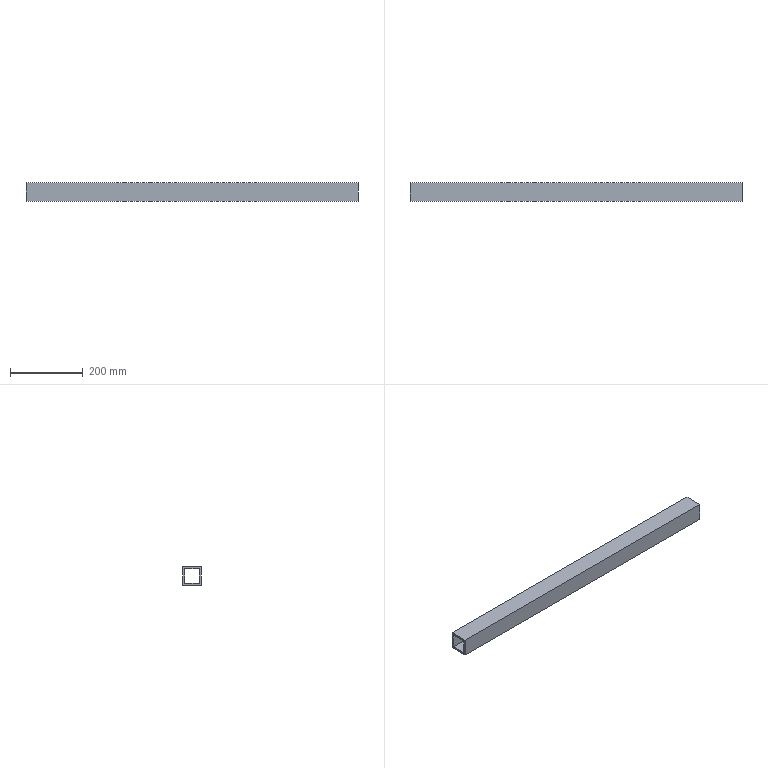Part | NX | features solid 2 | 1 solid | 10 faces | box 910 x 50 x 50 mm | volume 819000 mm3 | plane 10
STEP:
#1=CARTESIAN_POINT('',(-330.,45.,-270.));
#2=VERTEX_POINT('',#1);
#3=CARTESIAN_POINT('',(-330.,5.,-270.));
#4=VERTEX_POINT('',#3);
#5=CARTESIAN_POINT('',(-330.,0.,-270.));
#6=DIRECTION('',(0.,-1.,0.));
#7=VECTOR('',#6,1000.);
#8=LINE('',#5,#7);
#9=EDGE_CURVE('',#2,#4,#8,.T.);
#10=ORIENTED_EDGE('',*,*,#9,.F.);
#11=CARTESIAN_POINT('',(-330.,45.,-230.));
#12=VERTEX_POINT('',#11);
#13=CARTESIAN_POINT('',(-330.,45.,-275.));
#14=DIRECTION('',(0.,0.,-1.));
#15=VECTOR('',#14,1000.);
#16=LINE('',#13,#15);
#17=EDGE_CURVE('',#12,#2,#16,.T.);
#18=ORIENTED_EDGE('',*,*,#17,.F.);
#19=CARTESIAN_POINT('',(-330.,5.,-230.));
#20=VERTEX_POINT('',#19);
#21=CARTESIAN_POINT('',(-330.,0.,-230.));
#22=DIRECTION('',(0.,1.,0.));
#23=VECTOR('',#22,1000.);
#24=LINE('',#21,#23);
#25=EDGE_CURVE('',#20,#12,#24,.T.);
#26=ORIENTED_EDGE('',*,*,#25,.F.);
#27=CARTESIAN_POINT('',(-330.,5.,-275.));
#28=DIRECTION('',(0.,0.,1.));
#29=VECTOR('',#28,1000.);
#30=LINE('',#27,#29);
#31=EDGE_CURVE('',#4,#20,#30,.T.);
#32=ORIENTED_EDGE('',*,*,#31,.F.);
#33=EDGE_LOOP('',(#10,#18,#26,#32));
#34=FACE_BOUND('',#33,.T.);
#35=CARTESIAN_POINT('',(-330.,0.,-225.));
#36=VERTEX_POINT('',#35);
#37=CARTESIAN_POINT('',(-330.,50.,-225.));
#38=VERTEX_POINT('',#37);
#39=CARTESIAN_POINT('',(-330.,0.,-225.));
#40=DIRECTION('',(0.,1.,0.));
#41=VECTOR('',#40,1000.);
#42=LINE('',#39,#41);
#43=EDGE_CURVE('',#36,#38,#42,.T.);
#44=ORIENTED_EDGE('',*,*,#43,.T.);
#45=CARTESIAN_POINT('',(-330.,50.,-275.));
#46=VERTEX_POINT('',#45);
#47=CARTESIAN_POINT('',(-330.,50.,-275.));
#48=DIRECTION('',(0.,0.,-1.));
#49=VECTOR('',#48,1000.);
#50=LINE('',#47,#49);
#51=EDGE_CURVE('',#38,#46,#50,.T.);
#52=ORIENTED_EDGE('',*,*,#51,.T.);
#53=CARTESIAN_POINT('',(-330.,0.,-275.));
#54=VERTEX_POINT('',#53);
#55=CARTESIAN_POINT('',(-330.,0.,-275.));
#56=DIRECTION('',(0.,-1.,0.));
#57=VECTOR('',#56,1000.);
#58=LINE('',#55,#57);
#59=EDGE_CURVE('',#46,#54,#58,.T.);
#60=ORIENTED_EDGE('',*,*,#59,.T.);
#61=CARTESIAN_POINT('',(-330.,0.,-275.));
#62=DIRECTION('',(0.,0.,1.));
#63=VECTOR('',#62,1000.);
#64=LINE('',#61,#63);
#65=EDGE_CURVE('',#54,#36,#64,.T.);
#66=ORIENTED_EDGE('',*,*,#65,.T.);
#67=EDGE_LOOP('',(#44,#52,#60,#66));
#68=FACE_BOUND('',#67,.T.);
#69=CARTESIAN_POINT('',(-330.,0.,-275.));
#70=DIRECTION('',(1.,0.,0.));
#71=DIRECTION('',(0.,-1.,0.));
#72=AXIS2_PLACEMENT_3D('',#69,#70,#71);
#73=PLANE('',#72);
#74=ADVANCED_FACE('',(#34,#68),#73,.F.);
#75=CARTESIAN_POINT('',(580.,0.,-275.));
#76=VERTEX_POINT('',#75);
#77=CARTESIAN_POINT('',(-360.,0.,-275.));
#78=DIRECTION('',(1.,0.,0.));
#79=VECTOR('',#78,1000.);
#80=LINE('',#77,#79);
#81=EDGE_CURVE('',#54,#76,#80,.T.);
#82=ORIENTED_EDGE('',*,*,#81,.T.);
#83=CARTESIAN_POINT('',(580.,0.,-225.));
#84=VERTEX_POINT('',#83);
#85=CARTESIAN_POINT('',(580.,0.,-275.));
#86=DIRECTION('',(0.,0.,-1.));
#87=VECTOR('',#86,1000.);
#88=LINE('',#85,#87);
#89=EDGE_CURVE('',#84,#76,#88,.T.);
#90=ORIENTED_EDGE('',*,*,#89,.F.);
#91=CARTESIAN_POINT('',(-360.,0.,-225.));
#92=DIRECTION('',(-1.,0.,0.));
#93=VECTOR('',#92,1000.);
#94=LINE('',#91,#93);
#95=EDGE_CURVE('',#84,#36,#94,.T.);
#96=ORIENTED_EDGE('',*,*,#95,.T.);
#97=ORIENTED_EDGE('',*,*,#65,.F.);
#98=EDGE_LOOP('',(#82,#90,#96,#97));
#99=FACE_BOUND('',#98,.T.);
#100=CARTESIAN_POINT('',(-360.,0.,-275.));
#101=DIRECTION('',(0.,1.,0.));
#102=DIRECTION('',(1.,0.,0.));
#103=AXIS2_PLACEMENT_3D('',#100,#101,#102);
#104=PLANE('',#103);
#105=ADVANCED_FACE('',(#99),#104,.F.);
#106=CARTESIAN_POINT('',(580.,50.,-275.));
#107=VERTEX_POINT('',#106);
#108=CARTESIAN_POINT('',(-360.,50.,-275.));
#109=DIRECTION('',(1.,0.,0.));
#110=VECTOR('',#109,1000.);
#111=LINE('',#108,#110);
#112=EDGE_CURVE('',#46,#107,#111,.T.);
#113=ORIENTED_EDGE('',*,*,#112,.T.);
#114=CARTESIAN_POINT('',(580.,0.,-275.));
#115=DIRECTION('',(0.,1.,0.));
#116=VECTOR('',#115,1000.);
#117=LINE('',#114,#116);
#118=EDGE_CURVE('',#76,#107,#117,.T.);
#119=ORIENTED_EDGE('',*,*,#118,.F.);
#120=ORIENTED_EDGE('',*,*,#81,.F.);
#121=ORIENTED_EDGE('',*,*,#59,.F.);
#122=EDGE_LOOP('',(#113,#119,#120,#121));
#123=FACE_BOUND('',#122,.T.);
#124=CARTESIAN_POINT('',(-360.,0.,-275.));
#125=DIRECTION('',(0.,0.,1.));
#126=DIRECTION('',(0.,-1.,0.));
#127=AXIS2_PLACEMENT_3D('',#124,#125,#126);
#128=PLANE('',#127);
#129=ADVANCED_FACE('',(#123),#128,.F.);
#130=CARTESIAN_POINT('',(580.,50.,-225.));
#131=VERTEX_POINT('',#130);
#132=CARTESIAN_POINT('',(-360.,50.,-225.));
#133=DIRECTION('',(1.,0.,0.));
#134=VECTOR('',#133,1000.);
#135=LINE('',#132,#134);
#136=EDGE_CURVE('',#38,#131,#135,.T.);
#137=ORIENTED_EDGE('',*,*,#136,.T.);
#138=CARTESIAN_POINT('',(580.,50.,-225.));
#139=DIRECTION('',(0.,0.,1.));
#140=VECTOR('',#139,1000.);
#141=LINE('',#138,#140);
#142=EDGE_CURVE('',#107,#131,#141,.T.);
#143=ORIENTED_EDGE('',*,*,#142,.F.);
#144=ORIENTED_EDGE('',*,*,#112,.F.);
#145=ORIENTED_EDGE('',*,*,#51,.F.);
#146=EDGE_LOOP('',(#137,#143,#144,#145));
#147=FACE_BOUND('',#146,.T.);
#148=CARTESIAN_POINT('',(-360.,50.,-225.));
#149=DIRECTION('',(0.,-1.,0.));
#150=DIRECTION('',(-1.,0.,0.));
#151=AXIS2_PLACEMENT_3D('',#148,#149,#150);
#152=PLANE('',#151);
#153=ADVANCED_FACE('',(#147),#152,.F.);
#154=ORIENTED_EDGE('',*,*,#95,.F.);
#155=CARTESIAN_POINT('',(580.,0.,-225.));
#156=DIRECTION('',(0.,-1.,0.));
#157=VECTOR('',#156,1000.);
#158=LINE('',#155,#157);
#159=EDGE_CURVE('',#131,#84,#158,.T.);
#160=ORIENTED_EDGE('',*,*,#159,.F.);
#161=ORIENTED_EDGE('',*,*,#136,.F.);
#162=ORIENTED_EDGE('',*,*,#43,.F.);
#163=EDGE_LOOP('',(#154,#160,#161,#162));
#164=FACE_BOUND('',#163,.T.);
#165=CARTESIAN_POINT('',(580.,0.,-225.));
#166=DIRECTION('',(0.,0.,-1.));
#167=DIRECTION('',(-1.,0.,0.));
#168=AXIS2_PLACEMENT_3D('',#165,#166,#167);
#169=PLANE('',#168);
#170=ADVANCED_FACE('',(#164),#169,.F.);
#171=CARTESIAN_POINT('',(580.,45.,-270.));
#172=VERTEX_POINT('',#171);
#173=CARTESIAN_POINT('',(580.,5.,-270.));
#174=VERTEX_POINT('',#173);
#175=CARTESIAN_POINT('',(580.,0.,-270.));
#176=DIRECTION('',(0.,-1.,0.));
#177=VECTOR('',#176,1000.);
#178=LINE('',#175,#177);
#179=EDGE_CURVE('',#172,#174,#178,.T.);
#180=ORIENTED_EDGE('',*,*,#179,.F.);
#181=CARTESIAN_POINT('',(-360.,45.,-270.));
#182=DIRECTION('',(1.,0.,0.));
#183=VECTOR('',#182,1000.);
#184=LINE('',#181,#183);
#185=EDGE_CURVE('',#2,#172,#184,.T.);
#186=ORIENTED_EDGE('',*,*,#185,.F.);
#187=ORIENTED_EDGE('',*,*,#9,.T.);
#188=CARTESIAN_POINT('',(-360.,5.,-270.));
#189=DIRECTION('',(-1.,0.,0.));
#190=VECTOR('',#189,1000.);
#191=LINE('',#188,#190);
#192=EDGE_CURVE('',#174,#4,#191,.T.);
#193=ORIENTED_EDGE('',*,*,#192,.F.);
#194=EDGE_LOOP('',(#180,#186,#187,#193));
#195=FACE_BOUND('',#194,.T.);
#196=CARTESIAN_POINT('',(-360.,45.,-270.));
#197=DIRECTION('',(0.,0.,1.));
#198=DIRECTION('',(0.,-1.,0.));
#199=AXIS2_PLACEMENT_3D('',#196,#197,#198);
#200=PLANE('',#199);
#201=ADVANCED_FACE('',(#195),#200,.T.);
#202=CARTESIAN_POINT('',(580.,5.,-230.));
#203=VERTEX_POINT('',#202);
#204=CARTESIAN_POINT('',(580.,5.,-275.));
#205=DIRECTION('',(0.,0.,1.));
#206=VECTOR('',#205,1000.);
#207=LINE('',#204,#206);
#208=EDGE_CURVE('',#174,#203,#207,.T.);
#209=ORIENTED_EDGE('',*,*,#208,.F.);
#210=ORIENTED_EDGE('',*,*,#192,.T.);
#211=ORIENTED_EDGE('',*,*,#31,.T.);
#212=CARTESIAN_POINT('',(580.,5.,-230.));
#213=DIRECTION('',(-1.,0.,0.));
#214=VECTOR('',#213,1000.);
#215=LINE('',#212,#214);
#216=EDGE_CURVE('',#203,#20,#215,.T.);
#217=ORIENTED_EDGE('',*,*,#216,.F.);
#218=EDGE_LOOP('',(#209,#210,#211,#217));
#219=FACE_BOUND('',#218,.T.);
#220=CARTESIAN_POINT('',(580.,5.,-270.));
#221=DIRECTION('',(0.,1.,0.));
#222=DIRECTION('',(1.,0.,0.));
#223=AXIS2_PLACEMENT_3D('',#220,#221,#222);
#224=PLANE('',#223);
#225=ADVANCED_FACE('',(#219),#224,.T.);
#226=CARTESIAN_POINT('',(580.,45.,-230.));
#227=VERTEX_POINT('',#226);
#228=CARTESIAN_POINT('',(580.,0.,-230.));
#229=DIRECTION('',(0.,1.,0.));
#230=VECTOR('',#229,1000.);
#231=LINE('',#228,#230);
#232=EDGE_CURVE('',#203,#227,#231,.T.);
#233=ORIENTED_EDGE('',*,*,#232,.F.);
#234=ORIENTED_EDGE('',*,*,#216,.T.);
#235=ORIENTED_EDGE('',*,*,#25,.T.);
#236=CARTESIAN_POINT('',(580.,45.,-230.));
#237=DIRECTION('',(-1.,0.,0.));
#238=VECTOR('',#237,1000.);
#239=LINE('',#236,#238);
#240=EDGE_CURVE('',#227,#12,#239,.T.);
#241=ORIENTED_EDGE('',*,*,#240,.F.);
#242=EDGE_LOOP('',(#233,#234,#235,#241));
#243=FACE_BOUND('',#242,.T.);
#244=CARTESIAN_POINT('',(580.,5.,-230.));
#245=DIRECTION('',(0.,0.,-1.));
#246=DIRECTION('',(-1.,0.,0.));
#247=AXIS2_PLACEMENT_3D('',#244,#245,#246);
#248=PLANE('',#247);
#249=ADVANCED_FACE('',(#243),#248,.T.);
#250=CARTESIAN_POINT('',(580.,45.,-275.));
#251=DIRECTION('',(0.,0.,-1.));
#252=VECTOR('',#251,1000.);
#253=LINE('',#250,#252);
#254=EDGE_CURVE('',#227,#172,#253,.T.);
#255=ORIENTED_EDGE('',*,*,#254,.F.);
#256=ORIENTED_EDGE('',*,*,#240,.T.);
#257=ORIENTED_EDGE('',*,*,#17,.T.);
#258=ORIENTED_EDGE('',*,*,#185,.T.);
#259=EDGE_LOOP('',(#255,#256,#257,#258));
#260=FACE_BOUND('',#259,.T.);
#261=CARTESIAN_POINT('',(-360.,45.,-230.));
#262=DIRECTION('',(0.,-1.,0.));
#263=DIRECTION('',(-1.,0.,0.));
#264=AXIS2_PLACEMENT_3D('',#261,#262,#263);
#265=PLANE('',#264);
#266=ADVANCED_FACE('',(#260),#265,.T.);
#267=ORIENTED_EDGE('',*,*,#232,.T.);
#268=ORIENTED_EDGE('',*,*,#254,.T.);
#269=ORIENTED_EDGE('',*,*,#179,.T.);
#270=ORIENTED_EDGE('',*,*,#208,.T.);
#271=EDGE_LOOP('',(#267,#268,#269,#270));
#272=FACE_BOUND('',#271,.T.);
#273=ORIENTED_EDGE('',*,*,#142,.T.);
#274=ORIENTED_EDGE('',*,*,#159,.T.);
#275=ORIENTED_EDGE('',*,*,#89,.T.);
#276=ORIENTED_EDGE('',*,*,#118,.T.);
#277=EDGE_LOOP('',(#273,#274,#275,#276));
#278=FACE_BOUND('',#277,.T.);
#279=CARTESIAN_POINT('',(580.,0.,-275.));
#280=DIRECTION('',(1.,0.,0.));
#281=DIRECTION('',(0.,-1.,0.));
#282=AXIS2_PLACEMENT_3D('',#279,#280,#281);
#283=PLANE('',#282);
#284=ADVANCED_FACE('',(#272,#278),#283,.T.);
#285=CLOSED_SHELL('',(#74,#105,#129,#153,#170,#201,#225,#249,#266,#284));
#286=MANIFOLD_SOLID_BREP('',#285);
#287=(LENGTH_UNIT()NAMED_UNIT(*)SI_UNIT(.MILLI.,.METRE.));
#288=UNCERTAINTY_MEASURE_WITH_UNIT(LENGTH_MEASURE(0.00001),#287,'','');
#289=(NAMED_UNIT(*)PLANE_ANGLE_UNIT()SI_UNIT($,.RADIAN.));
#290=(NAMED_UNIT(*)SI_UNIT($,.STERADIAN.)SOLID_ANGLE_UNIT());
#291=(GEOMETRIC_REPRESENTATION_CONTEXT(3)GLOBAL_UNCERTAINTY_ASSIGNED_CONTEXT((#288))GLOBAL_UNIT_ASSIGNED_CONTEXT((#287,#289,#290))REPRESENTATION_CONTEXT('',''));
#292=ADVANCED_BREP_SHAPE_REPRESENTATION('',(#286),#291);